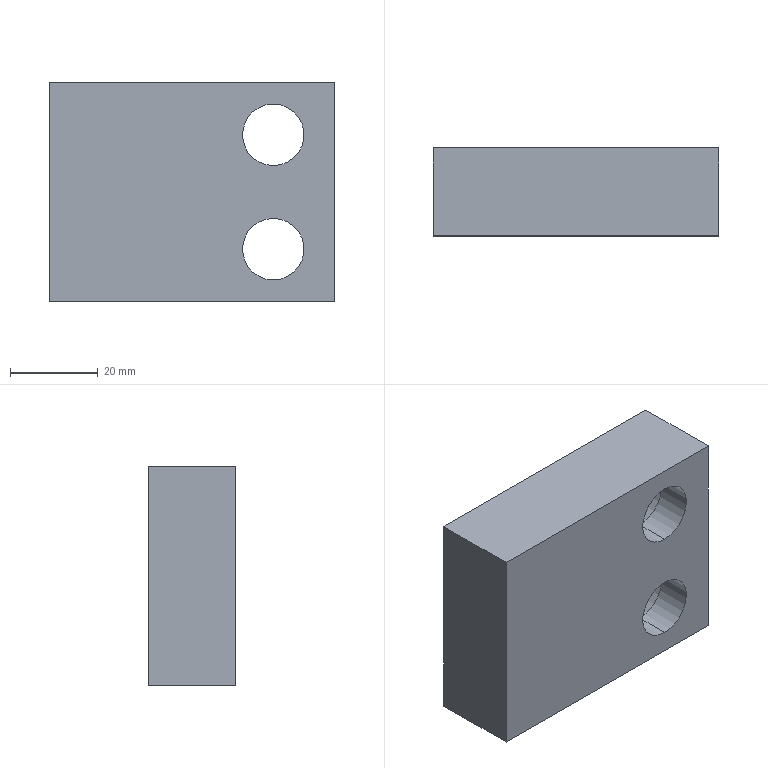Part | STEP file | OP10-026_stopper plate | 1 solid | 20 faces | box 65 x 20 x 50 mm | volume 54932 mm3 | cylinder 8 | plane 8 | cone 4 | commonest cylinder face diameters 14 x4 20 x4
STEP:
#1=CARTESIAN_POINT('',(0.,0.,0.));
#2=DIRECTION('',(0.,0.,1.));
#3=DIRECTION('',(1.,0.,0.));
#4=AXIS2_PLACEMENT_3D('',#1,#2,#3);
#5=CARTESIAN_POINT('',(18.5,19.,-3.));
#6=VERTEX_POINT('',#5);
#7=CARTESIAN_POINT('',(18.5,20.,-2.));
#8=VERTEX_POINT('',#7);
#9=CARTESIAN_POINT('',(18.5,19.,-3.));
#10=DIRECTION('',(0.,0.7071,0.7071));
#11=VECTOR('',#10,1.);
#12=LINE('',#9,#11);
#13=CARTESIAN_POINT('',(18.5,19.,-13.));
#14=DIRECTION('',(0.,1.,0.));
#15=DIRECTION('',(0.,0.,1.));
#16=AXIS2_PLACEMENT_3D('',#13,#14,#15);
#17=CONICAL_SURFACE('',#16,10.,0.7854);
#18=CARTESIAN_POINT('',(6.283,0.));
#19=DIRECTION('',(0.,1.));
#20=VECTOR('',#19,1.);
#21=LINE('',#18,#20);
#22=(GEOMETRIC_REPRESENTATION_CONTEXT(2)PARAMETRIC_REPRESENTATION_CONTEXT()REPRESENTATION_CONTEXT('',''));
#23=DEFINITIONAL_REPRESENTATION('',(#21),#22);
#24=PCURVE('',#17,#23);
#25=CARTESIAN_POINT('',(18.5,19.,-13.));
#26=DIRECTION('',(0.,1.,0.));
#27=DIRECTION('',(0.,0.,1.));
#28=AXIS2_PLACEMENT_3D('',#25,#26,#27);
#29=CONICAL_SURFACE('',#28,10.,0.7854);
#30=CARTESIAN_POINT('',(0.,0.));
#31=DIRECTION('',(0.,1.));
#32=VECTOR('',#31,1.);
#33=LINE('',#30,#32);
#34=(GEOMETRIC_REPRESENTATION_CONTEXT(2)PARAMETRIC_REPRESENTATION_CONTEXT()REPRESENTATION_CONTEXT('',''));
#35=DEFINITIONAL_REPRESENTATION('',(#33),#34);
#36=PCURVE('',#29,#35);
#37=SURFACE_CURVE('',#12,(#24,#36),.PCURVE_S1.);
#38=EDGE_CURVE('',#6,#8,#37,.T.);
#39=ORIENTED_EDGE('',*,*,#38,.T.);
#40=CARTESIAN_POINT('',(18.5,20.,-24.));
#41=VERTEX_POINT('',#40);
#42=CARTESIAN_POINT('',(18.5,20.,-13.));
#43=DIRECTION('',(0.,-1.,0.));
#44=DIRECTION('',(0.,0.,-1.));
#45=AXIS2_PLACEMENT_3D('',#42,#43,#44);
#46=CIRCLE('',#45,11.);
#47=CARTESIAN_POINT('',(9.425,1.));
#48=DIRECTION('',(-1.,0.));
#49=VECTOR('',#48,1.);
#50=LINE('',#47,#49);
#51=(GEOMETRIC_REPRESENTATION_CONTEXT(2)PARAMETRIC_REPRESENTATION_CONTEXT()REPRESENTATION_CONTEXT('',''));
#52=DEFINITIONAL_REPRESENTATION('',(#50),#51);
#53=PCURVE('',#17,#52);
#54=CARTESIAN_POINT('',(0.,20.,0.));
#55=DIRECTION('',(0.,-1.,0.));
#56=DIRECTION('',(0.,0.,-1.));
#57=AXIS2_PLACEMENT_3D('',#54,#55,#56);
#58=PLANE('',#57);
#59=CARTESIAN_POINT('',(13.,18.5));
#60=DIRECTION('',(1.,0.));
#61=AXIS2_PLACEMENT_2D('',#59,#60);
#62=CIRCLE('',#61,11.);
#63=(GEOMETRIC_REPRESENTATION_CONTEXT(2)PARAMETRIC_REPRESENTATION_CONTEXT()REPRESENTATION_CONTEXT('',''));
#64=DEFINITIONAL_REPRESENTATION('',(#62),#63);
#65=PCURVE('',#58,#64);
#66=SURFACE_CURVE('',#46,(#53,#65),.PCURVE_S1.);
#67=EDGE_CURVE('',#8,#41,#66,.T.);
#68=ORIENTED_EDGE('',*,*,#67,.T.);
#69=CARTESIAN_POINT('',(18.5,19.,-23.));
#70=VERTEX_POINT('',#69);
#71=CARTESIAN_POINT('',(18.5,19.,-23.));
#72=DIRECTION('',(0.,0.7071,-0.7071));
#73=VECTOR('',#72,1.);
#74=LINE('',#71,#73);
#75=CARTESIAN_POINT('',(3.142,0.));
#76=DIRECTION('',(0.,1.));
#77=VECTOR('',#76,1.);
#78=LINE('',#75,#77);
#79=(GEOMETRIC_REPRESENTATION_CONTEXT(2)PARAMETRIC_REPRESENTATION_CONTEXT()REPRESENTATION_CONTEXT('',''));
#80=DEFINITIONAL_REPRESENTATION('',(#78),#79);
#81=PCURVE('',#17,#80);
#82=CARTESIAN_POINT('',(3.142,0.));
#83=DIRECTION('',(0.,1.));
#84=VECTOR('',#83,1.);
#85=LINE('',#82,#84);
#86=(GEOMETRIC_REPRESENTATION_CONTEXT(2)PARAMETRIC_REPRESENTATION_CONTEXT()REPRESENTATION_CONTEXT('',''));
#87=DEFINITIONAL_REPRESENTATION('',(#85),#86);
#88=PCURVE('',#29,#87);
#89=SURFACE_CURVE('',#74,(#81,#88),.PCURVE_S1.);
#90=EDGE_CURVE('',#70,#41,#89,.T.);
#91=ORIENTED_EDGE('',*,*,#90,.F.);
#92=CARTESIAN_POINT('',(18.5,19.,-13.));
#93=DIRECTION('',(0.,1.,0.));
#94=DIRECTION('',(0.,0.,-1.));
#95=AXIS2_PLACEMENT_3D('',#92,#93,#94);
#96=CIRCLE('',#95,10.);
#97=CARTESIAN_POINT('',(3.142,0.));
#98=DIRECTION('',(1.,0.));
#99=VECTOR('',#98,1.);
#100=LINE('',#97,#99);
#101=(GEOMETRIC_REPRESENTATION_CONTEXT(2)PARAMETRIC_REPRESENTATION_CONTEXT()REPRESENTATION_CONTEXT('',''));
#102=DEFINITIONAL_REPRESENTATION('',(#100),#101);
#103=PCURVE('',#17,#102);
#104=CARTESIAN_POINT('',(18.5,20.,-13.));
#105=DIRECTION('',(0.,1.,0.));
#106=DIRECTION('',(0.,0.,1.));
#107=AXIS2_PLACEMENT_3D('',#104,#105,#106);
#108=CYLINDRICAL_SURFACE('',#107,10.);
#109=CARTESIAN_POINT('',(3.142,-1.));
#110=DIRECTION('',(1.,0.));
#111=VECTOR('',#110,1.);
#112=LINE('',#109,#111);
#113=(GEOMETRIC_REPRESENTATION_CONTEXT(2)PARAMETRIC_REPRESENTATION_CONTEXT()REPRESENTATION_CONTEXT('',''));
#114=DEFINITIONAL_REPRESENTATION('',(#112),#113);
#115=PCURVE('',#108,#114);
#116=SURFACE_CURVE('',#96,(#103,#115),.PCURVE_S1.);
#117=EDGE_CURVE('',#70,#6,#116,.T.);
#118=ORIENTED_EDGE('',*,*,#117,.T.);
#119=EDGE_LOOP('',(#39,#68,#91,#118));
#120=FACE_BOUND('',#119,.F.);
#121=ADVANCED_FACE('',(#120),#17,.F.);
#122=CARTESIAN_POINT('',(18.5,19.,23.));
#123=VERTEX_POINT('',#122);
#124=CARTESIAN_POINT('',(18.5,20.,24.));
#125=VERTEX_POINT('',#124);
#126=CARTESIAN_POINT('',(18.5,19.,23.));
#127=DIRECTION('',(0.,0.7071,0.7071));
#128=VECTOR('',#127,1.);
#129=LINE('',#126,#128);
#130=CARTESIAN_POINT('',(18.5,19.,13.));
#131=DIRECTION('',(0.,1.,0.));
#132=DIRECTION('',(0.,0.,1.));
#133=AXIS2_PLACEMENT_3D('',#130,#131,#132);
#134=CONICAL_SURFACE('',#133,10.,0.7854);
#135=CARTESIAN_POINT('',(6.283,0.));
#136=DIRECTION('',(0.,1.));
#137=VECTOR('',#136,1.);
#138=LINE('',#135,#137);
#139=(GEOMETRIC_REPRESENTATION_CONTEXT(2)PARAMETRIC_REPRESENTATION_CONTEXT()REPRESENTATION_CONTEXT('',''));
#140=DEFINITIONAL_REPRESENTATION('',(#138),#139);
#141=PCURVE('',#134,#140);
#142=CARTESIAN_POINT('',(18.5,19.,13.));
#143=DIRECTION('',(0.,1.,0.));
#144=DIRECTION('',(0.,0.,1.));
#145=AXIS2_PLACEMENT_3D('',#142,#143,#144);
#146=CONICAL_SURFACE('',#145,10.,0.7854);
#147=CARTESIAN_POINT('',(0.,0.));
#148=DIRECTION('',(0.,1.));
#149=VECTOR('',#148,1.);
#150=LINE('',#147,#149);
#151=(GEOMETRIC_REPRESENTATION_CONTEXT(2)PARAMETRIC_REPRESENTATION_CONTEXT()REPRESENTATION_CONTEXT('',''));
#152=DEFINITIONAL_REPRESENTATION('',(#150),#151);
#153=PCURVE('',#146,#152);
#154=SURFACE_CURVE('',#129,(#141,#153),.PCURVE_S1.);
#155=EDGE_CURVE('',#123,#125,#154,.T.);
#156=ORIENTED_EDGE('',*,*,#155,.T.);
#157=CARTESIAN_POINT('',(18.5,20.,2.));
#158=VERTEX_POINT('',#157);
#159=CARTESIAN_POINT('',(18.5,20.,13.));
#160=DIRECTION('',(0.,-1.,0.));
#161=DIRECTION('',(0.,0.,-1.));
#162=AXIS2_PLACEMENT_3D('',#159,#160,#161);
#163=CIRCLE('',#162,11.);
#164=CARTESIAN_POINT('',(9.425,1.));
#165=DIRECTION('',(-1.,0.));
#166=VECTOR('',#165,1.);
#167=LINE('',#164,#166);
#168=(GEOMETRIC_REPRESENTATION_CONTEXT(2)PARAMETRIC_REPRESENTATION_CONTEXT()REPRESENTATION_CONTEXT('',''));
#169=DEFINITIONAL_REPRESENTATION('',(#167),#168);
#170=PCURVE('',#134,#169);
#171=CARTESIAN_POINT('',(-13.,18.5));
#172=DIRECTION('',(1.,0.));
#173=AXIS2_PLACEMENT_2D('',#171,#172);
#174=CIRCLE('',#173,11.);
#175=(GEOMETRIC_REPRESENTATION_CONTEXT(2)PARAMETRIC_REPRESENTATION_CONTEXT()REPRESENTATION_CONTEXT('',''));
#176=DEFINITIONAL_REPRESENTATION('',(#174),#175);
#177=PCURVE('',#58,#176);
#178=SURFACE_CURVE('',#163,(#170,#177),.PCURVE_S1.);
#179=EDGE_CURVE('',#125,#158,#178,.T.);
#180=ORIENTED_EDGE('',*,*,#179,.T.);
#181=CARTESIAN_POINT('',(18.5,19.,3.));
#182=VERTEX_POINT('',#181);
#183=CARTESIAN_POINT('',(18.5,19.,3.));
#184=DIRECTION('',(0.,0.7071,-0.7071));
#185=VECTOR('',#184,1.);
#186=LINE('',#183,#185);
#187=CARTESIAN_POINT('',(3.142,0.));
#188=DIRECTION('',(0.,1.));
#189=VECTOR('',#188,1.);
#190=LINE('',#187,#189);
#191=(GEOMETRIC_REPRESENTATION_CONTEXT(2)PARAMETRIC_REPRESENTATION_CONTEXT()REPRESENTATION_CONTEXT('',''));
#192=DEFINITIONAL_REPRESENTATION('',(#190),#191);
#193=PCURVE('',#134,#192);
#194=CARTESIAN_POINT('',(3.142,0.));
#195=DIRECTION('',(0.,1.));
#196=VECTOR('',#195,1.);
#197=LINE('',#194,#196);
#198=(GEOMETRIC_REPRESENTATION_CONTEXT(2)PARAMETRIC_REPRESENTATION_CONTEXT()REPRESENTATION_CONTEXT('',''));
#199=DEFINITIONAL_REPRESENTATION('',(#197),#198);
#200=PCURVE('',#146,#199);
#201=SURFACE_CURVE('',#186,(#193,#200),.PCURVE_S1.);
#202=EDGE_CURVE('',#182,#158,#201,.T.);
#203=ORIENTED_EDGE('',*,*,#202,.F.);
#204=CARTESIAN_POINT('',(18.5,19.,13.));
#205=DIRECTION('',(0.,1.,0.));
#206=DIRECTION('',(0.,0.,-1.));
#207=AXIS2_PLACEMENT_3D('',#204,#205,#206);
#208=CIRCLE('',#207,10.);
#209=CARTESIAN_POINT('',(3.142,0.));
#210=DIRECTION('',(1.,0.));
#211=VECTOR('',#210,1.);
#212=LINE('',#209,#211);
#213=(GEOMETRIC_REPRESENTATION_CONTEXT(2)PARAMETRIC_REPRESENTATION_CONTEXT()REPRESENTATION_CONTEXT('',''));
#214=DEFINITIONAL_REPRESENTATION('',(#212),#213);
#215=PCURVE('',#134,#214);
#216=CARTESIAN_POINT('',(18.5,20.,13.));
#217=DIRECTION('',(0.,1.,0.));
#218=DIRECTION('',(0.,0.,1.));
#219=AXIS2_PLACEMENT_3D('',#216,#217,#218);
#220=CYLINDRICAL_SURFACE('',#219,10.);
#221=CARTESIAN_POINT('',(3.142,-1.));
#222=DIRECTION('',(1.,0.));
#223=VECTOR('',#222,1.);
#224=LINE('',#221,#223);
#225=(GEOMETRIC_REPRESENTATION_CONTEXT(2)PARAMETRIC_REPRESENTATION_CONTEXT()REPRESENTATION_CONTEXT('',''));
#226=DEFINITIONAL_REPRESENTATION('',(#224),#225);
#227=PCURVE('',#220,#226);
#228=SURFACE_CURVE('',#208,(#215,#227),.PCURVE_S1.);
#229=EDGE_CURVE('',#182,#123,#228,.T.);
#230=ORIENTED_EDGE('',*,*,#229,.T.);
#231=EDGE_LOOP('',(#156,#180,#203,#230));
#232=FACE_BOUND('',#231,.F.);
#233=ADVANCED_FACE('',(#232),#134,.F.);
#234=CARTESIAN_POINT('',(18.5,8.,23.));
#235=VERTEX_POINT('',#234);
#236=CARTESIAN_POINT('',(18.5,20.,23.));
#237=DIRECTION('',(0.,1.,0.));
#238=VECTOR('',#237,1.);
#239=LINE('',#236,#238);
#240=CARTESIAN_POINT('',(6.283,0.));
#241=DIRECTION('',(0.,1.));
#242=VECTOR('',#241,1.);
#243=LINE('',#240,#242);
#244=(GEOMETRIC_REPRESENTATION_CONTEXT(2)PARAMETRIC_REPRESENTATION_CONTEXT()REPRESENTATION_CONTEXT('',''));
#245=DEFINITIONAL_REPRESENTATION('',(#243),#244);
#246=PCURVE('',#220,#245);
#247=CARTESIAN_POINT('',(18.5,20.,13.));
#248=DIRECTION('',(0.,1.,0.));
#249=DIRECTION('',(0.,0.,1.));
#250=AXIS2_PLACEMENT_3D('',#247,#248,#249);
#251=CYLINDRICAL_SURFACE('',#250,10.);
#252=CARTESIAN_POINT('',(0.,0.));
#253=DIRECTION('',(0.,1.));
#254=VECTOR('',#253,1.);
#255=LINE('',#252,#254);
#256=(GEOMETRIC_REPRESENTATION_CONTEXT(2)PARAMETRIC_REPRESENTATION_CONTEXT()REPRESENTATION_CONTEXT('',''));
#257=DEFINITIONAL_REPRESENTATION('',(#255),#256);
#258=PCURVE('',#251,#257);
#259=SURFACE_CURVE('',#239,(#246,#258),.PCURVE_S1.);
#260=EDGE_CURVE('',#235,#123,#259,.T.);
#261=ORIENTED_EDGE('',*,*,#260,.T.);
#262=ORIENTED_EDGE('',*,*,#229,.F.);
#263=CARTESIAN_POINT('',(18.5,8.,3.));
#264=VERTEX_POINT('',#263);
#265=CARTESIAN_POINT('',(18.5,20.,3.));
#266=DIRECTION('',(0.,1.,0.));
#267=VECTOR('',#266,1.);
#268=LINE('',#265,#267);
#269=CARTESIAN_POINT('',(3.142,0.));
#270=DIRECTION('',(0.,1.));
#271=VECTOR('',#270,1.);
#272=LINE('',#269,#271);
#273=(GEOMETRIC_REPRESENTATION_CONTEXT(2)PARAMETRIC_REPRESENTATION_CONTEXT()REPRESENTATION_CONTEXT('',''));
#274=DEFINITIONAL_REPRESENTATION('',(#272),#273);
#275=PCURVE('',#220,#274);
#276=CARTESIAN_POINT('',(3.142,0.));
#277=DIRECTION('',(0.,1.));
#278=VECTOR('',#277,1.);
#279=LINE('',#276,#278);
#280=(GEOMETRIC_REPRESENTATION_CONTEXT(2)PARAMETRIC_REPRESENTATION_CONTEXT()REPRESENTATION_CONTEXT('',''));
#281=DEFINITIONAL_REPRESENTATION('',(#279),#280);
#282=PCURVE('',#251,#281);
#283=SURFACE_CURVE('',#268,(#275,#282),.PCURVE_S1.);
#284=EDGE_CURVE('',#264,#182,#283,.T.);
#285=ORIENTED_EDGE('',*,*,#284,.F.);
#286=CARTESIAN_POINT('',(18.5,8.,13.));
#287=DIRECTION('',(0.,1.,0.));
#288=DIRECTION('',(0.,0.,1.));
#289=AXIS2_PLACEMENT_3D('',#286,#287,#288);
#290=CIRCLE('',#289,10.);
#291=CARTESIAN_POINT('',(0.,-12.));
#292=DIRECTION('',(1.,0.));
#293=VECTOR('',#292,1.);
#294=LINE('',#291,#293);
#295=(GEOMETRIC_REPRESENTATION_CONTEXT(2)PARAMETRIC_REPRESENTATION_CONTEXT()REPRESENTATION_CONTEXT('',''));
#296=DEFINITIONAL_REPRESENTATION('',(#294),#295);
#297=PCURVE('',#220,#296);
#298=CARTESIAN_POINT('',(25.5,8.,13.));
#299=DIRECTION('',(0.,-1.,0.));
#300=DIRECTION('',(0.,0.,-1.));
#301=AXIS2_PLACEMENT_3D('',#298,#299,#300);
#302=PLANE('',#301);
#303=CARTESIAN_POINT('',(-10.,-7.));
#304=CARTESIAN_POINT('',(-10.,10.321));
#305=CARTESIAN_POINT('',(5.,1.66));
#306=CARTESIAN_POINT('',(20.,-7.));
#307=CARTESIAN_POINT('',(5.,-15.66));
#308=CARTESIAN_POINT('',(-10.,-24.321));
#309=CARTESIAN_POINT('',(-10.,-7.));
#310=(BOUNDED_CURVE()B_SPLINE_CURVE(2,(#303,#304,#305,#306,#307,#308,#309),.UNSPECIFIED.,.T.,.F.)B_SPLINE_CURVE_WITH_KNOTS((1,2,2,2,2,1),(-2.094,0.,2.094,4.189,6.283,8.378),.UNSPECIFIED.)CURVE()GEOMETRIC_REPRESENTATION_ITEM()RATIONAL_B_SPLINE_CURVE((1.,0.5,1.,0.5,1.,0.5,1.))REPRESENTATION_ITEM(''));
#311=(GEOMETRIC_REPRESENTATION_CONTEXT(2)PARAMETRIC_REPRESENTATION_CONTEXT()REPRESENTATION_CONTEXT('',''));
#312=DEFINITIONAL_REPRESENTATION('',(#310),#311);
#313=PCURVE('',#302,#312);
#314=SURFACE_CURVE('',#290,(#297,#313),.PCURVE_S1.);
#315=EDGE_CURVE('',#264,#235,#314,.T.);
#316=ORIENTED_EDGE('',*,*,#315,.T.);
#317=EDGE_LOOP('',(#261,#262,#285,#316));
#318=FACE_BOUND('',#317,.F.);
#319=ADVANCED_FACE('',(#318),#220,.F.);
#320=CARTESIAN_POINT('',(18.5,0.,20.));
#321=VERTEX_POINT('',#320);
#322=CARTESIAN_POINT('',(18.5,8.,20.));
#323=VERTEX_POINT('',#322);
#324=CARTESIAN_POINT('',(18.5,20.,20.));
#325=DIRECTION('',(0.,1.,0.));
#326=VECTOR('',#325,1.);
#327=LINE('',#324,#326);
#328=CARTESIAN_POINT('',(18.5,20.,13.));
#329=DIRECTION('',(0.,1.,0.));
#330=DIRECTION('',(0.,0.,1.));
#331=AXIS2_PLACEMENT_3D('',#328,#329,#330);
#332=CYLINDRICAL_SURFACE('',#331,7.);
#333=CARTESIAN_POINT('',(6.283,0.));
#334=DIRECTION('',(0.,1.));
#335=VECTOR('',#334,1.);
#336=LINE('',#333,#335);
#337=(GEOMETRIC_REPRESENTATION_CONTEXT(2)PARAMETRIC_REPRESENTATION_CONTEXT()REPRESENTATION_CONTEXT('',''));
#338=DEFINITIONAL_REPRESENTATION('',(#336),#337);
#339=PCURVE('',#332,#338);
#340=CARTESIAN_POINT('',(18.5,20.,13.));
#341=DIRECTION('',(0.,1.,0.));
#342=DIRECTION('',(0.,0.,1.));
#343=AXIS2_PLACEMENT_3D('',#340,#341,#342);
#344=CYLINDRICAL_SURFACE('',#343,7.);
#345=CARTESIAN_POINT('',(0.,0.));
#346=DIRECTION('',(0.,1.));
#347=VECTOR('',#346,1.);
#348=LINE('',#345,#347);
#349=(GEOMETRIC_REPRESENTATION_CONTEXT(2)PARAMETRIC_REPRESENTATION_CONTEXT()REPRESENTATION_CONTEXT('',''));
#350=DEFINITIONAL_REPRESENTATION('',(#348),#349);
#351=PCURVE('',#344,#350);
#352=SURFACE_CURVE('',#327,(#339,#351),.PCURVE_S1.);
#353=EDGE_CURVE('',#321,#323,#352,.T.);
#354=ORIENTED_EDGE('',*,*,#353,.T.);
#355=CARTESIAN_POINT('',(18.5,8.,6.));
#356=VERTEX_POINT('',#355);
#357=CARTESIAN_POINT('',(18.5,8.,13.));
#358=DIRECTION('',(0.,1.,0.));
#359=DIRECTION('',(0.,0.,1.));
#360=AXIS2_PLACEMENT_3D('',#357,#358,#359);
#361=CIRCLE('',#360,7.);
#362=CARTESIAN_POINT('',(0.,-12.));
#363=DIRECTION('',(1.,0.));
#364=VECTOR('',#363,1.);
#365=LINE('',#362,#364);
#366=(GEOMETRIC_REPRESENTATION_CONTEXT(2)PARAMETRIC_REPRESENTATION_CONTEXT()REPRESENTATION_CONTEXT('',''));
#367=DEFINITIONAL_REPRESENTATION('',(#365),#366);
#368=PCURVE('',#332,#367);
#369=CARTESIAN_POINT('',(-7.,-7.));
#370=CARTESIAN_POINT('',(-7.,5.124));
#371=CARTESIAN_POINT('',(3.5,-0.9378));
#372=CARTESIAN_POINT('',(14.,-7.));
#373=CARTESIAN_POINT('',(3.5,-13.062));
#374=CARTESIAN_POINT('',(-7.,-19.124));
#375=CARTESIAN_POINT('',(-7.,-7.));
#376=(BOUNDED_CURVE()B_SPLINE_CURVE(2,(#369,#370,#371,#372,#373,#374,#375),.UNSPECIFIED.,.T.,.F.)B_SPLINE_CURVE_WITH_KNOTS((1,2,2,2,2,1),(-2.094,0.,2.094,4.189,6.283,8.378),.UNSPECIFIED.)CURVE()GEOMETRIC_REPRESENTATION_ITEM()RATIONAL_B_SPLINE_CURVE((1.,0.5,1.,0.5,1.,0.5,1.))REPRESENTATION_ITEM(''));
#377=(GEOMETRIC_REPRESENTATION_CONTEXT(2)PARAMETRIC_REPRESENTATION_CONTEXT()REPRESENTATION_CONTEXT('',''));
#378=DEFINITIONAL_REPRESENTATION('',(#376),#377);
#379=PCURVE('',#302,#378);
#380=SURFACE_CURVE('',#361,(#368,#379),.PCURVE_S1.);
#381=EDGE_CURVE('',#356,#323,#380,.T.);
#382=ORIENTED_EDGE('',*,*,#381,.F.);
#383=CARTESIAN_POINT('',(18.5,0.,6.));
#384=VERTEX_POINT('',#383);
#385=CARTESIAN_POINT('',(18.5,20.,6.));
#386=DIRECTION('',(0.,1.,0.));
#387=VECTOR('',#386,1.);
#388=LINE('',#385,#387);
#389=CARTESIAN_POINT('',(3.142,0.));
#390=DIRECTION('',(0.,1.));
#391=VECTOR('',#390,1.);
#392=LINE('',#389,#391);
#393=(GEOMETRIC_REPRESENTATION_CONTEXT(2)PARAMETRIC_REPRESENTATION_CONTEXT()REPRESENTATION_CONTEXT('',''));
#394=DEFINITIONAL_REPRESENTATION('',(#392),#393);
#395=PCURVE('',#332,#394);
#396=CARTESIAN_POINT('',(3.142,0.));
#397=DIRECTION('',(0.,1.));
#398=VECTOR('',#397,1.);
#399=LINE('',#396,#398);
#400=(GEOMETRIC_REPRESENTATION_CONTEXT(2)PARAMETRIC_REPRESENTATION_CONTEXT()REPRESENTATION_CONTEXT('',''));
#401=DEFINITIONAL_REPRESENTATION('',(#399),#400);
#402=PCURVE('',#344,#401);
#403=SURFACE_CURVE('',#388,(#395,#402),.PCURVE_S1.);
#404=EDGE_CURVE('',#384,#356,#403,.T.);
#405=ORIENTED_EDGE('',*,*,#404,.F.);
#406=CARTESIAN_POINT('',(18.5,0.,13.));
#407=DIRECTION('',(0.,1.,0.));
#408=DIRECTION('',(0.,0.,1.));
#409=AXIS2_PLACEMENT_3D('',#406,#407,#408);
#410=CIRCLE('',#409,7.);
#411=CARTESIAN_POINT('',(0.,-20.));
#412=DIRECTION('',(1.,0.));
#413=VECTOR('',#412,1.);
#414=LINE('',#411,#413);
#415=(GEOMETRIC_REPRESENTATION_CONTEXT(2)PARAMETRIC_REPRESENTATION_CONTEXT()REPRESENTATION_CONTEXT('',''));
#416=DEFINITIONAL_REPRESENTATION('',(#414),#415);
#417=PCURVE('',#332,#416);
#418=CARTESIAN_POINT('',(0.,0.,0.));
#419=DIRECTION('',(0.,-1.,0.));
#420=DIRECTION('',(0.,0.,-1.));
#421=AXIS2_PLACEMENT_3D('',#418,#419,#420);
#422=PLANE('',#421);
#423=CARTESIAN_POINT('',(-20.,18.5));
#424=CARTESIAN_POINT('',(-20.,30.624));
#425=CARTESIAN_POINT('',(-9.5,24.562));
#426=CARTESIAN_POINT('',(1.,18.5));
#427=CARTESIAN_POINT('',(-9.5,12.438));
#428=CARTESIAN_POINT('',(-20.,6.376));
#429=CARTESIAN_POINT('',(-20.,18.5));
#430=(BOUNDED_CURVE()B_SPLINE_CURVE(2,(#423,#424,#425,#426,#427,#428,#429),.UNSPECIFIED.,.T.,.F.)B_SPLINE_CURVE_WITH_KNOTS((1,2,2,2,2,1),(-2.094,0.,2.094,4.189,6.283,8.378),.UNSPECIFIED.)CURVE()GEOMETRIC_REPRESENTATION_ITEM()RATIONAL_B_SPLINE_CURVE((1.,0.5,1.,0.5,1.,0.5,1.))REPRESENTATION_ITEM(''));
#431=(GEOMETRIC_REPRESENTATION_CONTEXT(2)PARAMETRIC_REPRESENTATION_CONTEXT()REPRESENTATION_CONTEXT('',''));
#432=DEFINITIONAL_REPRESENTATION('',(#430),#431);
#433=PCURVE('',#422,#432);
#434=SURFACE_CURVE('',#410,(#417,#433),.PCURVE_S1.);
#435=EDGE_CURVE('',#384,#321,#434,.T.);
#436=ORIENTED_EDGE('',*,*,#435,.T.);
#437=EDGE_LOOP('',(#354,#382,#405,#436));
#438=FACE_BOUND('',#437,.F.);
#439=ADVANCED_FACE('',(#438),#332,.F.);
#440=CARTESIAN_POINT('',(18.5,8.,-3.));
#441=VERTEX_POINT('',#440);
#442=CARTESIAN_POINT('',(18.5,20.,-3.));
#443=DIRECTION('',(0.,1.,0.));
#444=VECTOR('',#443,1.);
#445=LINE('',#442,#444);
#446=CARTESIAN_POINT('',(6.283,0.));
#447=DIRECTION('',(0.,1.));
#448=VECTOR('',#447,1.);
#449=LINE('',#446,#448);
#450=(GEOMETRIC_REPRESENTATION_CONTEXT(2)PARAMETRIC_REPRESENTATION_CONTEXT()REPRESENTATION_CONTEXT('',''));
#451=DEFINITIONAL_REPRESENTATION('',(#449),#450);
#452=PCURVE('',#108,#451);
#453=CARTESIAN_POINT('',(18.5,20.,-13.));
#454=DIRECTION('',(0.,1.,0.));
#455=DIRECTION('',(0.,0.,1.));
#456=AXIS2_PLACEMENT_3D('',#453,#454,#455);
#457=CYLINDRICAL_SURFACE('',#456,10.);
#458=CARTESIAN_POINT('',(0.,0.));
#459=DIRECTION('',(0.,1.));
#460=VECTOR('',#459,1.);
#461=LINE('',#458,#460);
#462=(GEOMETRIC_REPRESENTATION_CONTEXT(2)PARAMETRIC_REPRESENTATION_CONTEXT()REPRESENTATION_CONTEXT('',''));
#463=DEFINITIONAL_REPRESENTATION('',(#461),#462);
#464=PCURVE('',#457,#463);
#465=SURFACE_CURVE('',#445,(#452,#464),.PCURVE_S1.);
#466=EDGE_CURVE('',#441,#6,#465,.T.);
#467=ORIENTED_EDGE('',*,*,#466,.T.);
#468=ORIENTED_EDGE('',*,*,#117,.F.);
#469=CARTESIAN_POINT('',(18.5,8.,-23.));
#470=VERTEX_POINT('',#469);
#471=CARTESIAN_POINT('',(18.5,20.,-23.));
#472=DIRECTION('',(0.,1.,0.));
#473=VECTOR('',#472,1.);
#474=LINE('',#471,#473);
#475=CARTESIAN_POINT('',(3.142,0.));
#476=DIRECTION('',(0.,1.));
#477=VECTOR('',#476,1.);
#478=LINE('',#475,#477);
#479=(GEOMETRIC_REPRESENTATION_CONTEXT(2)PARAMETRIC_REPRESENTATION_CONTEXT()REPRESENTATION_CONTEXT('',''));
#480=DEFINITIONAL_REPRESENTATION('',(#478),#479);
#481=PCURVE('',#108,#480);
#482=CARTESIAN_POINT('',(3.142,0.));
#483=DIRECTION('',(0.,1.));
#484=VECTOR('',#483,1.);
#485=LINE('',#482,#484);
#486=(GEOMETRIC_REPRESENTATION_CONTEXT(2)PARAMETRIC_REPRESENTATION_CONTEXT()REPRESENTATION_CONTEXT('',''));
#487=DEFINITIONAL_REPRESENTATION('',(#485),#486);
#488=PCURVE('',#457,#487);
#489=SURFACE_CURVE('',#474,(#481,#488),.PCURVE_S1.);
#490=EDGE_CURVE('',#470,#70,#489,.T.);
#491=ORIENTED_EDGE('',*,*,#490,.F.);
#492=CARTESIAN_POINT('',(18.5,8.,-13.));
#493=DIRECTION('',(0.,1.,0.));
#494=DIRECTION('',(0.,0.,1.));
#495=AXIS2_PLACEMENT_3D('',#492,#493,#494);
#496=CIRCLE('',#495,10.);
#497=CARTESIAN_POINT('',(0.,-12.));
#498=DIRECTION('',(1.,0.));
#499=VECTOR('',#498,1.);
#500=LINE('',#497,#499);
#501=(GEOMETRIC_REPRESENTATION_CONTEXT(2)PARAMETRIC_REPRESENTATION_CONTEXT()REPRESENTATION_CONTEXT('',''));
#502=DEFINITIONAL_REPRESENTATION('',(#500),#501);
#503=PCURVE('',#108,#502);
#504=CARTESIAN_POINT('',(25.5,8.,-13.));
#505=DIRECTION('',(0.,-1.,0.));
#506=DIRECTION('',(0.,0.,-1.));
#507=AXIS2_PLACEMENT_3D('',#504,#505,#506);
#508=PLANE('',#507);
#509=CARTESIAN_POINT('',(-10.,-7.));
#510=CARTESIAN_POINT('',(-10.,10.321));
#511=CARTESIAN_POINT('',(5.,1.66));
#512=CARTESIAN_POINT('',(20.,-7.));
#513=CARTESIAN_POINT('',(5.,-15.66));
#514=CARTESIAN_POINT('',(-10.,-24.321));
#515=CARTESIAN_POINT('',(-10.,-7.));
#516=(BOUNDED_CURVE()B_SPLINE_CURVE(2,(#509,#510,#511,#512,#513,#514,#515),.UNSPECIFIED.,.T.,.F.)B_SPLINE_CURVE_WITH_KNOTS((1,2,2,2,2,1),(-2.094,0.,2.094,4.189,6.283,8.378),.UNSPECIFIED.)CURVE()GEOMETRIC_REPRESENTATION_ITEM()RATIONAL_B_SPLINE_CURVE((1.,0.5,1.,0.5,1.,0.5,1.))REPRESENTATION_ITEM(''));
#517=(GEOMETRIC_REPRESENTATION_CONTEXT(2)PARAMETRIC_REPRESENTATION_CONTEXT()REPRESENTATION_CONTEXT('',''));
#518=DEFINITIONAL_REPRESENTATION('',(#516),#517);
#519=PCURVE('',#508,#518);
#520=SURFACE_CURVE('',#496,(#503,#519),.PCURVE_S1.);
#521=EDGE_CURVE('',#470,#441,#520,.T.);
#522=ORIENTED_EDGE('',*,*,#521,.T.);
#523=EDGE_LOOP('',(#467,#468,#491,#522));
#524=FACE_BOUND('',#523,.F.);
#525=ADVANCED_FACE('',(#524),#108,.F.);
#526=CARTESIAN_POINT('',(18.5,0.,-6.));
#527=VERTEX_POINT('',#526);
#528=CARTESIAN_POINT('',(18.5,8.,-6.));
#529=VERTEX_POINT('',#528);
#530=CARTESIAN_POINT('',(18.5,20.,-6.));
#531=DIRECTION('',(0.,1.,0.));
#532=VECTOR('',#531,1.);
#533=LINE('',#530,#532);
#534=CARTESIAN_POINT('',(18.5,20.,-13.));
#535=DIRECTION('',(0.,1.,0.));
#536=DIRECTION('',(0.,0.,1.));
#537=AXIS2_PLACEMENT_3D('',#534,#535,#536);
#538=CYLINDRICAL_SURFACE('',#537,7.);
#539=CARTESIAN_POINT('',(6.283,0.));
#540=DIRECTION('',(0.,1.));
#541=VECTOR('',#540,1.);
#542=LINE('',#539,#541);
#543=(GEOMETRIC_REPRESENTATION_CONTEXT(2)PARAMETRIC_REPRESENTATION_CONTEXT()REPRESENTATION_CONTEXT('',''));
#544=DEFINITIONAL_REPRESENTATION('',(#542),#543);
#545=PCURVE('',#538,#544);
#546=CARTESIAN_POINT('',(18.5,20.,-13.));
#547=DIRECTION('',(0.,1.,0.));
#548=DIRECTION('',(0.,0.,1.));
#549=AXIS2_PLACEMENT_3D('',#546,#547,#548);
#550=CYLINDRICAL_SURFACE('',#549,7.);
#551=CARTESIAN_POINT('',(0.,0.));
#552=DIRECTION('',(0.,1.));
#553=VECTOR('',#552,1.);
#554=LINE('',#551,#553);
#555=(GEOMETRIC_REPRESENTATION_CONTEXT(2)PARAMETRIC_REPRESENTATION_CONTEXT()REPRESENTATION_CONTEXT('',''));
#556=DEFINITIONAL_REPRESENTATION('',(#554),#555);
#557=PCURVE('',#550,#556);
#558=SURFACE_CURVE('',#533,(#545,#557),.PCURVE_S1.);
#559=EDGE_CURVE('',#527,#529,#558,.T.);
#560=ORIENTED_EDGE('',*,*,#559,.T.);
#561=CARTESIAN_POINT('',(18.5,8.,-20.));
#562=VERTEX_POINT('',#561);
#563=CARTESIAN_POINT('',(18.5,8.,-13.));
#564=DIRECTION('',(0.,1.,0.));
#565=DIRECTION('',(0.,0.,1.));
#566=AXIS2_PLACEMENT_3D('',#563,#564,#565);
#567=CIRCLE('',#566,7.);
#568=CARTESIAN_POINT('',(0.,-12.));
#569=DIRECTION('',(1.,0.));
#570=VECTOR('',#569,1.);
#571=LINE('',#568,#570);
#572=(GEOMETRIC_REPRESENTATION_CONTEXT(2)PARAMETRIC_REPRESENTATION_CONTEXT()REPRESENTATION_CONTEXT('',''));
#573=DEFINITIONAL_REPRESENTATION('',(#571),#572);
#574=PCURVE('',#538,#573);
#575=CARTESIAN_POINT('',(-7.,-7.));
#576=CARTESIAN_POINT('',(-7.,5.124));
#577=CARTESIAN_POINT('',(3.5,-0.9378));
#578=CARTESIAN_POINT('',(14.,-7.));
#579=CARTESIAN_POINT('',(3.5,-13.062));
#580=CARTESIAN_POINT('',(-7.,-19.124));
#581=CARTESIAN_POINT('',(-7.,-7.));
#582=(BOUNDED_CURVE()B_SPLINE_CURVE(2,(#575,#576,#577,#578,#579,#580,#581),.UNSPECIFIED.,.T.,.F.)B_SPLINE_CURVE_WITH_KNOTS((1,2,2,2,2,1),(-2.094,0.,2.094,4.189,6.283,8.378),.UNSPECIFIED.)CURVE()GEOMETRIC_REPRESENTATION_ITEM()RATIONAL_B_SPLINE_CURVE((1.,0.5,1.,0.5,1.,0.5,1.))REPRESENTATION_ITEM(''));
#583=(GEOMETRIC_REPRESENTATION_CONTEXT(2)PARAMETRIC_REPRESENTATION_CONTEXT()REPRESENTATION_CONTEXT('',''));
#584=DEFINITIONAL_REPRESENTATION('',(#582),#583);
#585=PCURVE('',#508,#584);
#586=SURFACE_CURVE('',#567,(#574,#585),.PCURVE_S1.);
#587=EDGE_CURVE('',#562,#529,#586,.T.);
#588=ORIENTED_EDGE('',*,*,#587,.F.);
#589=CARTESIAN_POINT('',(18.5,0.,-20.));
#590=VERTEX_POINT('',#589);
#591=CARTESIAN_POINT('',(18.5,20.,-20.));
#592=DIRECTION('',(0.,1.,0.));
#593=VECTOR('',#592,1.);
#594=LINE('',#591,#593);
#595=CARTESIAN_POINT('',(3.142,0.));
#596=DIRECTION('',(0.,1.));
#597=VECTOR('',#596,1.);
#598=LINE('',#595,#597);
#599=(GEOMETRIC_REPRESENTATION_CONTEXT(2)PARAMETRIC_REPRESENTATION_CONTEXT()REPRESENTATION_CONTEXT('',''));
#600=DEFINITIONAL_REPRESENTATION('',(#598),#599);
#601=PCURVE('',#538,#600);
#602=CARTESIAN_POINT('',(3.142,0.));
#603=DIRECTION('',(0.,1.));
#604=VECTOR('',#603,1.);
#605=LINE('',#602,#604);
#606=(GEOMETRIC_REPRESENTATION_CONTEXT(2)PARAMETRIC_REPRESENTATION_CONTEXT()REPRESENTATION_CONTEXT('',''));
#607=DEFINITIONAL_REPRESENTATION('',(#605),#606);
#608=PCURVE('',#550,#607);
#609=SURFACE_CURVE('',#594,(#601,#608),.PCURVE_S1.);
#610=EDGE_CURVE('',#590,#562,#609,.T.);
#611=ORIENTED_EDGE('',*,*,#610,.F.);
#612=CARTESIAN_POINT('',(18.5,0.,-13.));
#613=DIRECTION('',(0.,1.,0.));
#614=DIRECTION('',(0.,0.,1.));
#615=AXIS2_PLACEMENT_3D('',#612,#613,#614);
#616=CIRCLE('',#615,7.);
#617=CARTESIAN_POINT('',(0.,-20.));
#618=DIRECTION('',(1.,0.));
#619=VECTOR('',#618,1.);
#620=LINE('',#617,#619);
#621=(GEOMETRIC_REPRESENTATION_CONTEXT(2)PARAMETRIC_REPRESENTATION_CONTEXT()REPRESENTATION_CONTEXT('',''));
#622=DEFINITIONAL_REPRESENTATION('',(#620),#621);
#623=PCURVE('',#538,#622);
#624=CARTESIAN_POINT('',(6.,18.5));
#625=CARTESIAN_POINT('',(6.,30.624));
#626=CARTESIAN_POINT('',(16.5,24.562));
#627=CARTESIAN_POINT('',(27.,18.5));
#628=CARTESIAN_POINT('',(16.5,12.438));
#629=CARTESIAN_POINT('',(6.,6.376));
#630=CARTESIAN_POINT('',(6.,18.5));
#631=(BOUNDED_CURVE()B_SPLINE_CURVE(2,(#624,#625,#626,#627,#628,#629,#630),.UNSPECIFIED.,.T.,.F.)B_SPLINE_CURVE_WITH_KNOTS((1,2,2,2,2,1),(-2.094,0.,2.094,4.189,6.283,8.378),.UNSPECIFIED.)CURVE()GEOMETRIC_REPRESENTATION_ITEM()RATIONAL_B_SPLINE_CURVE((1.,0.5,1.,0.5,1.,0.5,1.))REPRESENTATION_ITEM(''));
#632=(GEOMETRIC_REPRESENTATION_CONTEXT(2)PARAMETRIC_REPRESENTATION_CONTEXT()REPRESENTATION_CONTEXT('',''));
#633=DEFINITIONAL_REPRESENTATION('',(#631),#632);
#634=PCURVE('',#422,#633);
#635=SURFACE_CURVE('',#616,(#623,#634),.PCURVE_S1.);
#636=EDGE_CURVE('',#590,#527,#635,.T.);
#637=ORIENTED_EDGE('',*,*,#636,.T.);
#638=EDGE_LOOP('',(#560,#588,#611,#637));
#639=FACE_BOUND('',#638,.F.);
#640=ADVANCED_FACE('',(#639),#538,.F.);
#641=CARTESIAN_POINT('',(32.5,0.,25.));
#642=VERTEX_POINT('',#641);
#643=CARTESIAN_POINT('',(32.5,0.,-25.));
#644=VERTEX_POINT('',#643);
#645=CARTESIAN_POINT('',(32.5,0.,25.));
#646=DIRECTION('',(0.,0.,-1.));
#647=VECTOR('',#646,1.);
#648=LINE('',#645,#647);
#649=CARTESIAN_POINT('',(32.5,20.,25.));
#650=DIRECTION('',(-1.,0.,0.));
#651=DIRECTION('',(0.,0.,1.));
#652=AXIS2_PLACEMENT_3D('',#649,#650,#651);
#653=PLANE('',#652);
#654=CARTESIAN_POINT('',(0.,-20.));
#655=DIRECTION('',(-1.,0.));
#656=VECTOR('',#655,1.);
#657=LINE('',#654,#656);
#658=(GEOMETRIC_REPRESENTATION_CONTEXT(2)PARAMETRIC_REPRESENTATION_CONTEXT()REPRESENTATION_CONTEXT('',''));
#659=DEFINITIONAL_REPRESENTATION('',(#657),#658);
#660=PCURVE('',#653,#659);
#661=CARTESIAN_POINT('',(-25.,32.5));
#662=DIRECTION('',(1.,0.));
#663=VECTOR('',#662,1.);
#664=LINE('',#661,#663);
#665=(GEOMETRIC_REPRESENTATION_CONTEXT(2)PARAMETRIC_REPRESENTATION_CONTEXT()REPRESENTATION_CONTEXT('',''));
#666=DEFINITIONAL_REPRESENTATION('',(#664),#665);
#667=PCURVE('',#422,#666);
#668=SURFACE_CURVE('',#648,(#660,#667),.PCURVE_S1.);
#669=EDGE_CURVE('',#642,#644,#668,.T.);
#670=ORIENTED_EDGE('',*,*,#669,.T.);
#671=CARTESIAN_POINT('',(32.5,20.,-25.));
#672=VERTEX_POINT('',#671);
#673=CARTESIAN_POINT('',(32.5,20.,-25.));
#674=DIRECTION('',(0.,-1.,0.));
#675=VECTOR('',#674,1.);
#676=LINE('',#673,#675);
#677=CARTESIAN_POINT('',(-50.,0.));
#678=DIRECTION('',(0.,-1.));
#679=VECTOR('',#678,1.);
#680=LINE('',#677,#679);
#681=(GEOMETRIC_REPRESENTATION_CONTEXT(2)PARAMETRIC_REPRESENTATION_CONTEXT()REPRESENTATION_CONTEXT('',''));
#682=DEFINITIONAL_REPRESENTATION('',(#680),#681);
#683=PCURVE('',#653,#682);
#684=CARTESIAN_POINT('',(-32.5,20.,-25.));
#685=DIRECTION('',(0.,0.,1.));
#686=DIRECTION('',(1.,0.,0.));
#687=AXIS2_PLACEMENT_3D('',#684,#685,#686);
#688=PLANE('',#687);
#689=CARTESIAN_POINT('',(65.,0.));
#690=DIRECTION('',(0.,-1.));
#691=VECTOR('',#690,1.);
#692=LINE('',#689,#691);
#693=(GEOMETRIC_REPRESENTATION_CONTEXT(2)PARAMETRIC_REPRESENTATION_CONTEXT()REPRESENTATION_CONTEXT('',''));
#694=DEFINITIONAL_REPRESENTATION('',(#692),#693);
#695=PCURVE('',#688,#694);
#696=SURFACE_CURVE('',#676,(#683,#695),.PCURVE_S1.);
#697=EDGE_CURVE('',#672,#644,#696,.T.);
#698=ORIENTED_EDGE('',*,*,#697,.F.);
#699=CARTESIAN_POINT('',(32.5,20.,25.));
#700=VERTEX_POINT('',#699);
#701=CARTESIAN_POINT('',(32.5,20.,25.));
#702=DIRECTION('',(0.,0.,-1.));
#703=VECTOR('',#702,1.);
#704=LINE('',#701,#703);
#705=CARTESIAN_POINT('',(0.,0.));
#706=DIRECTION('',(-1.,0.));
#707=VECTOR('',#706,1.);
#708=LINE('',#705,#707);
#709=(GEOMETRIC_REPRESENTATION_CONTEXT(2)PARAMETRIC_REPRESENTATION_CONTEXT()REPRESENTATION_CONTEXT('',''));
#710=DEFINITIONAL_REPRESENTATION('',(#708),#709);
#711=PCURVE('',#653,#710);
#712=CARTESIAN_POINT('',(-25.,32.5));
#713=DIRECTION('',(1.,0.));
#714=VECTOR('',#713,1.);
#715=LINE('',#712,#714);
#716=(GEOMETRIC_REPRESENTATION_CONTEXT(2)PARAMETRIC_REPRESENTATION_CONTEXT()REPRESENTATION_CONTEXT('',''));
#717=DEFINITIONAL_REPRESENTATION('',(#715),#716);
#718=PCURVE('',#58,#717);
#719=SURFACE_CURVE('',#704,(#711,#718),.PCURVE_S1.);
#720=EDGE_CURVE('',#700,#672,#719,.T.);
#721=ORIENTED_EDGE('',*,*,#720,.F.);
#722=CARTESIAN_POINT('',(32.5,20.,25.));
#723=DIRECTION('',(0.,-1.,0.));
#724=VECTOR('',#723,1.);
#725=LINE('',#722,#724);
#726=CARTESIAN_POINT('',(0.,0.));
#727=DIRECTION('',(0.,-1.));
#728=VECTOR('',#727,1.);
#729=LINE('',#726,#728);
#730=(GEOMETRIC_REPRESENTATION_CONTEXT(2)PARAMETRIC_REPRESENTATION_CONTEXT()REPRESENTATION_CONTEXT('',''));
#731=DEFINITIONAL_REPRESENTATION('',(#729),#730);
#732=PCURVE('',#653,#731);
#733=CARTESIAN_POINT('',(-32.5,20.,25.));
#734=DIRECTION('',(0.,0.,-1.));
#735=DIRECTION('',(-1.,0.,0.));
#736=AXIS2_PLACEMENT_3D('',#733,#734,#735);
#737=PLANE('',#736);
#738=CARTESIAN_POINT('',(-65.,0.));
#739=DIRECTION('',(0.,-1.));
#740=VECTOR('',#739,1.);
#741=LINE('',#738,#740);
#742=(GEOMETRIC_REPRESENTATION_CONTEXT(2)PARAMETRIC_REPRESENTATION_CONTEXT()REPRESENTATION_CONTEXT('',''));
#743=DEFINITIONAL_REPRESENTATION('',(#741),#742);
#744=PCURVE('',#737,#743);
#745=SURFACE_CURVE('',#725,(#732,#744),.PCURVE_S1.);
#746=EDGE_CURVE('',#700,#642,#745,.T.);
#747=ORIENTED_EDGE('',*,*,#746,.T.);
#748=EDGE_LOOP('',(#670,#698,#721,#747));
#749=FACE_BOUND('',#748,.T.);
#750=ADVANCED_FACE('',(#749),#653,.F.);
#751=CARTESIAN_POINT('',(-32.5,0.,-25.));
#752=VERTEX_POINT('',#751);
#753=CARTESIAN_POINT('',(-32.5,0.,-25.));
#754=DIRECTION('',(-1.,0.,0.));
#755=VECTOR('',#754,1.);
#756=LINE('',#753,#755);
#757=CARTESIAN_POINT('',(0.,-20.));
#758=DIRECTION('',(-1.,0.));
#759=VECTOR('',#758,1.);
#760=LINE('',#757,#759);
#761=(GEOMETRIC_REPRESENTATION_CONTEXT(2)PARAMETRIC_REPRESENTATION_CONTEXT()REPRESENTATION_CONTEXT('',''));
#762=DEFINITIONAL_REPRESENTATION('',(#760),#761);
#763=PCURVE('',#688,#762);
#764=CARTESIAN_POINT('',(25.,-32.5));
#765=DIRECTION('',(0.,-1.));
#766=VECTOR('',#765,1.);
#767=LINE('',#764,#766);
#768=(GEOMETRIC_REPRESENTATION_CONTEXT(2)PARAMETRIC_REPRESENTATION_CONTEXT()REPRESENTATION_CONTEXT('',''));
#769=DEFINITIONAL_REPRESENTATION('',(#767),#768);
#770=PCURVE('',#422,#769);
#771=SURFACE_CURVE('',#756,(#763,#770),.PCURVE_S1.);
#772=EDGE_CURVE('',#644,#752,#771,.T.);
#773=ORIENTED_EDGE('',*,*,#772,.T.);
#774=CARTESIAN_POINT('',(-32.5,20.,-25.));
#775=VERTEX_POINT('',#774);
#776=CARTESIAN_POINT('',(-32.5,20.,-25.));
#777=DIRECTION('',(0.,-1.,0.));
#778=VECTOR('',#777,1.);
#779=LINE('',#776,#778);
#780=CARTESIAN_POINT('',(0.,0.));
#781=DIRECTION('',(0.,-1.));
#782=VECTOR('',#781,1.);
#783=LINE('',#780,#782);
#784=(GEOMETRIC_REPRESENTATION_CONTEXT(2)PARAMETRIC_REPRESENTATION_CONTEXT()REPRESENTATION_CONTEXT('',''));
#785=DEFINITIONAL_REPRESENTATION('',(#783),#784);
#786=PCURVE('',#688,#785);
#787=CARTESIAN_POINT('',(-32.5,20.,25.));
#788=DIRECTION('',(1.,0.,0.));
#789=DIRECTION('',(0.,0.,-1.));
#790=AXIS2_PLACEMENT_3D('',#787,#788,#789);
#791=PLANE('',#790);
#792=CARTESIAN_POINT('',(50.,0.));
#793=DIRECTION('',(0.,-1.));
#794=VECTOR('',#793,1.);
#795=LINE('',#792,#794);
#796=(GEOMETRIC_REPRESENTATION_CONTEXT(2)PARAMETRIC_REPRESENTATION_CONTEXT()REPRESENTATION_CONTEXT('',''));
#797=DEFINITIONAL_REPRESENTATION('',(#795),#796);
#798=PCURVE('',#791,#797);
#799=SURFACE_CURVE('',#779,(#786,#798),.PCURVE_S1.);
#800=EDGE_CURVE('',#775,#752,#799,.T.);
#801=ORIENTED_EDGE('',*,*,#800,.F.);
#802=CARTESIAN_POINT('',(-32.5,20.,-25.));
#803=DIRECTION('',(-1.,0.,0.));
#804=VECTOR('',#803,1.);
#805=LINE('',#802,#804);
#806=CARTESIAN_POINT('',(0.,0.));
#807=DIRECTION('',(-1.,0.));
#808=VECTOR('',#807,1.);
#809=LINE('',#806,#808);
#810=(GEOMETRIC_REPRESENTATION_CONTEXT(2)PARAMETRIC_REPRESENTATION_CONTEXT()REPRESENTATION_CONTEXT('',''));
#811=DEFINITIONAL_REPRESENTATION('',(#809),#810);
#812=PCURVE('',#688,#811);
#813=CARTESIAN_POINT('',(25.,-32.5));
#814=DIRECTION('',(0.,-1.));
#815=VECTOR('',#814,1.);
#816=LINE('',#813,#815);
#817=(GEOMETRIC_REPRESENTATION_CONTEXT(2)PARAMETRIC_REPRESENTATION_CONTEXT()REPRESENTATION_CONTEXT('',''));
#818=DEFINITIONAL_REPRESENTATION('',(#816),#817);
#819=PCURVE('',#58,#818);
#820=SURFACE_CURVE('',#805,(#812,#819),.PCURVE_S1.);
#821=EDGE_CURVE('',#672,#775,#820,.T.);
#822=ORIENTED_EDGE('',*,*,#821,.F.);
#823=ORIENTED_EDGE('',*,*,#697,.T.);
#824=EDGE_LOOP('',(#773,#801,#822,#823));
#825=FACE_BOUND('',#824,.T.);
#826=ADVANCED_FACE('',(#825),#688,.F.);
#827=CARTESIAN_POINT('',(-32.5,0.,25.));
#828=VERTEX_POINT('',#827);
#829=CARTESIAN_POINT('',(-32.5,0.,25.));
#830=DIRECTION('',(0.,0.,1.));
#831=VECTOR('',#830,1.);
#832=LINE('',#829,#831);
#833=CARTESIAN_POINT('',(0.,-20.));
#834=DIRECTION('',(-1.,0.));
#835=VECTOR('',#834,1.);
#836=LINE('',#833,#835);
#837=(GEOMETRIC_REPRESENTATION_CONTEXT(2)PARAMETRIC_REPRESENTATION_CONTEXT()REPRESENTATION_CONTEXT('',''));
#838=DEFINITIONAL_REPRESENTATION('',(#836),#837);
#839=PCURVE('',#791,#838);
#840=CARTESIAN_POINT('',(-25.,-32.5));
#841=DIRECTION('',(-1.,0.));
#842=VECTOR('',#841,1.);
#843=LINE('',#840,#842);
#844=(GEOMETRIC_REPRESENTATION_CONTEXT(2)PARAMETRIC_REPRESENTATION_CONTEXT()REPRESENTATION_CONTEXT('',''));
#845=DEFINITIONAL_REPRESENTATION('',(#843),#844);
#846=PCURVE('',#422,#845);
#847=SURFACE_CURVE('',#832,(#839,#846),.PCURVE_S1.);
#848=EDGE_CURVE('',#752,#828,#847,.T.);
#849=ORIENTED_EDGE('',*,*,#848,.T.);
#850=CARTESIAN_POINT('',(-32.5,20.,25.));
#851=VERTEX_POINT('',#850);
#852=CARTESIAN_POINT('',(-32.5,20.,25.));
#853=DIRECTION('',(0.,-1.,0.));
#854=VECTOR('',#853,1.);
#855=LINE('',#852,#854);
#856=CARTESIAN_POINT('',(0.,0.));
#857=DIRECTION('',(0.,-1.));
#858=VECTOR('',#857,1.);
#859=LINE('',#856,#858);
#860=(GEOMETRIC_REPRESENTATION_CONTEXT(2)PARAMETRIC_REPRESENTATION_CONTEXT()REPRESENTATION_CONTEXT('',''));
#861=DEFINITIONAL_REPRESENTATION('',(#859),#860);
#862=PCURVE('',#791,#861);
#863=CARTESIAN_POINT('',(0.,0.));
#864=DIRECTION('',(0.,-1.));
#865=VECTOR('',#864,1.);
#866=LINE('',#863,#865);
#867=(GEOMETRIC_REPRESENTATION_CONTEXT(2)PARAMETRIC_REPRESENTATION_CONTEXT()REPRESENTATION_CONTEXT('',''));
#868=DEFINITIONAL_REPRESENTATION('',(#866),#867);
#869=PCURVE('',#737,#868);
#870=SURFACE_CURVE('',#855,(#862,#869),.PCURVE_S1.);
#871=EDGE_CURVE('',#851,#828,#870,.T.);
#872=ORIENTED_EDGE('',*,*,#871,.F.);
#873=CARTESIAN_POINT('',(-32.5,20.,25.));
#874=DIRECTION('',(0.,0.,1.));
#875=VECTOR('',#874,1.);
#876=LINE('',#873,#875);
#877=CARTESIAN_POINT('',(0.,0.));
#878=DIRECTION('',(-1.,0.));
#879=VECTOR('',#878,1.);
#880=LINE('',#877,#879);
#881=(GEOMETRIC_REPRESENTATION_CONTEXT(2)PARAMETRIC_REPRESENTATION_CONTEXT()REPRESENTATION_CONTEXT('',''));
#882=DEFINITIONAL_REPRESENTATION('',(#880),#881);
#883=PCURVE('',#791,#882);
#884=CARTESIAN_POINT('',(-25.,-32.5));
#885=DIRECTION('',(-1.,0.));
#886=VECTOR('',#885,1.);
#887=LINE('',#884,#886);
#888=(GEOMETRIC_REPRESENTATION_CONTEXT(2)PARAMETRIC_REPRESENTATION_CONTEXT()REPRESENTATION_CONTEXT('',''));
#889=DEFINITIONAL_REPRESENTATION('',(#887),#888);
#890=PCURVE('',#58,#889);
#891=SURFACE_CURVE('',#876,(#883,#890),.PCURVE_S1.);
#892=EDGE_CURVE('',#775,#851,#891,.T.);
#893=ORIENTED_EDGE('',*,*,#892,.F.);
#894=ORIENTED_EDGE('',*,*,#800,.T.);
#895=EDGE_LOOP('',(#849,#872,#893,#894));
#896=FACE_BOUND('',#895,.T.);
#897=ADVANCED_FACE('',(#896),#791,.F.);
#898=CARTESIAN_POINT('',(-32.5,0.,25.));
#899=DIRECTION('',(1.,0.,0.));
#900=VECTOR('',#899,1.);
#901=LINE('',#898,#900);
#902=CARTESIAN_POINT('',(0.,-20.));
#903=DIRECTION('',(-1.,0.));
#904=VECTOR('',#903,1.);
#905=LINE('',#902,#904);
#906=(GEOMETRIC_REPRESENTATION_CONTEXT(2)PARAMETRIC_REPRESENTATION_CONTEXT()REPRESENTATION_CONTEXT('',''));
#907=DEFINITIONAL_REPRESENTATION('',(#905),#906);
#908=PCURVE('',#737,#907);
#909=CARTESIAN_POINT('',(-25.,-32.5));
#910=DIRECTION('',(0.,1.));
#911=VECTOR('',#910,1.);
#912=LINE('',#909,#911);
#913=(GEOMETRIC_REPRESENTATION_CONTEXT(2)PARAMETRIC_REPRESENTATION_CONTEXT()REPRESENTATION_CONTEXT('',''));
#914=DEFINITIONAL_REPRESENTATION('',(#912),#913);
#915=PCURVE('',#422,#914);
#916=SURFACE_CURVE('',#901,(#908,#915),.PCURVE_S1.);
#917=EDGE_CURVE('',#828,#642,#916,.T.);
#918=ORIENTED_EDGE('',*,*,#917,.T.);
#919=ORIENTED_EDGE('',*,*,#746,.F.);
#920=CARTESIAN_POINT('',(-32.5,20.,25.));
#921=DIRECTION('',(1.,0.,0.));
#922=VECTOR('',#921,1.);
#923=LINE('',#920,#922);
#924=CARTESIAN_POINT('',(0.,0.));
#925=DIRECTION('',(-1.,0.));
#926=VECTOR('',#925,1.);
#927=LINE('',#924,#926);
#928=(GEOMETRIC_REPRESENTATION_CONTEXT(2)PARAMETRIC_REPRESENTATION_CONTEXT()REPRESENTATION_CONTEXT('',''));
#929=DEFINITIONAL_REPRESENTATION('',(#927),#928);
#930=PCURVE('',#737,#929);
#931=CARTESIAN_POINT('',(-25.,-32.5));
#932=DIRECTION('',(0.,1.));
#933=VECTOR('',#932,1.);
#934=LINE('',#931,#933);
#935=(GEOMETRIC_REPRESENTATION_CONTEXT(2)PARAMETRIC_REPRESENTATION_CONTEXT()REPRESENTATION_CONTEXT('',''));
#936=DEFINITIONAL_REPRESENTATION('',(#934),#935);
#937=PCURVE('',#58,#936);
#938=SURFACE_CURVE('',#923,(#930,#937),.PCURVE_S1.);
#939=EDGE_CURVE('',#851,#700,#938,.T.);
#940=ORIENTED_EDGE('',*,*,#939,.F.);
#941=ORIENTED_EDGE('',*,*,#871,.T.);
#942=EDGE_LOOP('',(#918,#919,#940,#941));
#943=FACE_BOUND('',#942,.T.);
#944=ADVANCED_FACE('',(#943),#737,.F.);
#945=ORIENTED_EDGE('',*,*,#179,.T.);
#946=CARTESIAN_POINT('',(18.5,20.,13.));
#947=DIRECTION('',(0.,-1.,0.));
#948=DIRECTION('',(0.,0.,-1.));
#949=AXIS2_PLACEMENT_3D('',#946,#947,#948);
#950=CIRCLE('',#949,11.);
#951=CARTESIAN_POINT('',(-13.,18.5));
#952=DIRECTION('',(1.,0.));
#953=AXIS2_PLACEMENT_2D('',#951,#952);
#954=CIRCLE('',#953,11.);
#955=(GEOMETRIC_REPRESENTATION_CONTEXT(2)PARAMETRIC_REPRESENTATION_CONTEXT()REPRESENTATION_CONTEXT('',''));
#956=DEFINITIONAL_REPRESENTATION('',(#954),#955);
#957=PCURVE('',#58,#956);
#958=CARTESIAN_POINT('',(3.142,1.));
#959=DIRECTION('',(-1.,0.));
#960=VECTOR('',#959,1.);
#961=LINE('',#958,#960);
#962=(GEOMETRIC_REPRESENTATION_CONTEXT(2)PARAMETRIC_REPRESENTATION_CONTEXT()REPRESENTATION_CONTEXT('',''));
#963=DEFINITIONAL_REPRESENTATION('',(#961),#962);
#964=PCURVE('',#146,#963);
#965=SURFACE_CURVE('',#950,(#957,#964),.PCURVE_S1.);
#966=EDGE_CURVE('',#158,#125,#965,.T.);
#967=ORIENTED_EDGE('',*,*,#966,.T.);
#968=EDGE_LOOP('',(#945,#967));
#969=FACE_BOUND('',#968,.T.);
#970=ORIENTED_EDGE('',*,*,#67,.T.);
#971=CARTESIAN_POINT('',(18.5,20.,-13.));
#972=DIRECTION('',(0.,-1.,0.));
#973=DIRECTION('',(0.,0.,-1.));
#974=AXIS2_PLACEMENT_3D('',#971,#972,#973);
#975=CIRCLE('',#974,11.);
#976=CARTESIAN_POINT('',(13.,18.5));
#977=DIRECTION('',(1.,0.));
#978=AXIS2_PLACEMENT_2D('',#976,#977);
#979=CIRCLE('',#978,11.);
#980=(GEOMETRIC_REPRESENTATION_CONTEXT(2)PARAMETRIC_REPRESENTATION_CONTEXT()REPRESENTATION_CONTEXT('',''));
#981=DEFINITIONAL_REPRESENTATION('',(#979),#980);
#982=PCURVE('',#58,#981);
#983=CARTESIAN_POINT('',(3.142,1.));
#984=DIRECTION('',(-1.,0.));
#985=VECTOR('',#984,1.);
#986=LINE('',#983,#985);
#987=(GEOMETRIC_REPRESENTATION_CONTEXT(2)PARAMETRIC_REPRESENTATION_CONTEXT()REPRESENTATION_CONTEXT('',''));
#988=DEFINITIONAL_REPRESENTATION('',(#986),#987);
#989=PCURVE('',#29,#988);
#990=SURFACE_CURVE('',#975,(#982,#989),.PCURVE_S1.);
#991=EDGE_CURVE('',#41,#8,#990,.T.);
#992=ORIENTED_EDGE('',*,*,#991,.T.);
#993=EDGE_LOOP('',(#970,#992));
#994=FACE_BOUND('',#993,.T.);
#995=ORIENTED_EDGE('',*,*,#720,.T.);
#996=ORIENTED_EDGE('',*,*,#821,.T.);
#997=ORIENTED_EDGE('',*,*,#892,.T.);
#998=ORIENTED_EDGE('',*,*,#939,.T.);
#999=EDGE_LOOP('',(#995,#996,#997,#998));
#1000=FACE_BOUND('',#999,.T.);
#1001=ADVANCED_FACE('',(#969,#994,#1000),#58,.F.);
#1002=CARTESIAN_POINT('',(18.5,0.,13.));
#1003=DIRECTION('',(0.,1.,0.));
#1004=DIRECTION('',(0.,0.,1.));
#1005=AXIS2_PLACEMENT_3D('',#1002,#1003,#1004);
#1006=CIRCLE('',#1005,7.);
#1007=CARTESIAN_POINT('',(-20.,18.5));
#1008=CARTESIAN_POINT('',(-20.,30.624));
#1009=CARTESIAN_POINT('',(-9.5,24.562));
#1010=CARTESIAN_POINT('',(1.,18.5));
#1011=CARTESIAN_POINT('',(-9.5,12.438));
#1012=CARTESIAN_POINT('',(-20.,6.376));
#1013=CARTESIAN_POINT('',(-20.,18.5));
#1014=(BOUNDED_CURVE()B_SPLINE_CURVE(2,(#1007,#1008,#1009,#1010,#1011,#1012,#1013),.UNSPECIFIED.,.T.,.F.)B_SPLINE_CURVE_WITH_KNOTS((1,2,2,2,2,1),(-2.094,0.,2.094,4.189,6.283,8.378),.UNSPECIFIED.)CURVE()GEOMETRIC_REPRESENTATION_ITEM()RATIONAL_B_SPLINE_CURVE((1.,0.5,1.,0.5,1.,0.5,1.))REPRESENTATION_ITEM(''));
#1015=(GEOMETRIC_REPRESENTATION_CONTEXT(2)PARAMETRIC_REPRESENTATION_CONTEXT()REPRESENTATION_CONTEXT('',''));
#1016=DEFINITIONAL_REPRESENTATION('',(#1014),#1015);
#1017=PCURVE('',#422,#1016);
#1018=CARTESIAN_POINT('',(0.,-20.));
#1019=DIRECTION('',(1.,0.));
#1020=VECTOR('',#1019,1.);
#1021=LINE('',#1018,#1020);
#1022=(GEOMETRIC_REPRESENTATION_CONTEXT(2)PARAMETRIC_REPRESENTATION_CONTEXT()REPRESENTATION_CONTEXT('',''));
#1023=DEFINITIONAL_REPRESENTATION('',(#1021),#1022);
#1024=PCURVE('',#344,#1023);
#1025=SURFACE_CURVE('',#1006,(#1017,#1024),.PCURVE_S1.);
#1026=EDGE_CURVE('',#321,#384,#1025,.T.);
#1027=ORIENTED_EDGE('',*,*,#1026,.T.);
#1028=ORIENTED_EDGE('',*,*,#435,.T.);
#1029=EDGE_LOOP('',(#1027,#1028));
#1030=FACE_BOUND('',#1029,.T.);
#1031=CARTESIAN_POINT('',(18.5,0.,-13.));
#1032=DIRECTION('',(0.,1.,0.));
#1033=DIRECTION('',(0.,0.,1.));
#1034=AXIS2_PLACEMENT_3D('',#1031,#1032,#1033);
#1035=CIRCLE('',#1034,7.);
#1036=CARTESIAN_POINT('',(6.,18.5));
#1037=CARTESIAN_POINT('',(6.,30.624));
#1038=CARTESIAN_POINT('',(16.5,24.562));
#1039=CARTESIAN_POINT('',(27.,18.5));
#1040=CARTESIAN_POINT('',(16.5,12.438));
#1041=CARTESIAN_POINT('',(6.,6.376));
#1042=CARTESIAN_POINT('',(6.,18.5));
#1043=(BOUNDED_CURVE()B_SPLINE_CURVE(2,(#1036,#1037,#1038,#1039,#1040,#1041,#1042),.UNSPECIFIED.,.T.,.F.)B_SPLINE_CURVE_WITH_KNOTS((1,2,2,2,2,1),(-2.094,0.,2.094,4.189,6.283,8.378),.UNSPECIFIED.)CURVE()GEOMETRIC_REPRESENTATION_ITEM()RATIONAL_B_SPLINE_CURVE((1.,0.5,1.,0.5,1.,0.5,1.))REPRESENTATION_ITEM(''));
#1044=(GEOMETRIC_REPRESENTATION_CONTEXT(2)PARAMETRIC_REPRESENTATION_CONTEXT()REPRESENTATION_CONTEXT('',''));
#1045=DEFINITIONAL_REPRESENTATION('',(#1043),#1044);
#1046=PCURVE('',#422,#1045);
#1047=CARTESIAN_POINT('',(0.,-20.));
#1048=DIRECTION('',(1.,0.));
#1049=VECTOR('',#1048,1.);
#1050=LINE('',#1047,#1049);
#1051=(GEOMETRIC_REPRESENTATION_CONTEXT(2)PARAMETRIC_REPRESENTATION_CONTEXT()REPRESENTATION_CONTEXT('',''));
#1052=DEFINITIONAL_REPRESENTATION('',(#1050),#1051);
#1053=PCURVE('',#550,#1052);
#1054=SURFACE_CURVE('',#1035,(#1046,#1053),.PCURVE_S1.);
#1055=EDGE_CURVE('',#527,#590,#1054,.T.);
#1056=ORIENTED_EDGE('',*,*,#1055,.T.);
#1057=ORIENTED_EDGE('',*,*,#636,.T.);
#1058=EDGE_LOOP('',(#1056,#1057));
#1059=FACE_BOUND('',#1058,.T.);
#1060=ORIENTED_EDGE('',*,*,#669,.F.);
#1061=ORIENTED_EDGE('',*,*,#917,.F.);
#1062=ORIENTED_EDGE('',*,*,#848,.F.);
#1063=ORIENTED_EDGE('',*,*,#772,.F.);
#1064=EDGE_LOOP('',(#1060,#1061,#1062,#1063));
#1065=FACE_BOUND('',#1064,.T.);
#1066=ADVANCED_FACE('',(#1030,#1059,#1065),#422,.T.);
#1067=CARTESIAN_POINT('',(18.5,8.,-13.));
#1068=DIRECTION('',(0.,1.,0.));
#1069=DIRECTION('',(0.,0.,1.));
#1070=AXIS2_PLACEMENT_3D('',#1067,#1068,#1069);
#1071=CIRCLE('',#1070,7.);
#1072=CARTESIAN_POINT('',(0.,-12.));
#1073=DIRECTION('',(1.,0.));
#1074=VECTOR('',#1073,1.);
#1075=LINE('',#1072,#1074);
#1076=(GEOMETRIC_REPRESENTATION_CONTEXT(2)PARAMETRIC_REPRESENTATION_CONTEXT()REPRESENTATION_CONTEXT('',''));
#1077=DEFINITIONAL_REPRESENTATION('',(#1075),#1076);
#1078=PCURVE('',#550,#1077);
#1079=CARTESIAN_POINT('',(-7.,-7.));
#1080=CARTESIAN_POINT('',(-7.,5.124));
#1081=CARTESIAN_POINT('',(3.5,-0.9378));
#1082=CARTESIAN_POINT('',(14.,-7.));
#1083=CARTESIAN_POINT('',(3.5,-13.062));
#1084=CARTESIAN_POINT('',(-7.,-19.124));
#1085=CARTESIAN_POINT('',(-7.,-7.));
#1086=(BOUNDED_CURVE()B_SPLINE_CURVE(2,(#1079,#1080,#1081,#1082,#1083,#1084,#1085),.UNSPECIFIED.,.T.,.F.)B_SPLINE_CURVE_WITH_KNOTS((1,2,2,2,2,1),(-2.094,0.,2.094,4.189,6.283,8.378),.UNSPECIFIED.)CURVE()GEOMETRIC_REPRESENTATION_ITEM()RATIONAL_B_SPLINE_CURVE((1.,0.5,1.,0.5,1.,0.5,1.))REPRESENTATION_ITEM(''));
#1087=(GEOMETRIC_REPRESENTATION_CONTEXT(2)PARAMETRIC_REPRESENTATION_CONTEXT()REPRESENTATION_CONTEXT('',''));
#1088=DEFINITIONAL_REPRESENTATION('',(#1086),#1087);
#1089=PCURVE('',#508,#1088);
#1090=SURFACE_CURVE('',#1071,(#1078,#1089),.PCURVE_S1.);
#1091=EDGE_CURVE('',#529,#562,#1090,.T.);
#1092=ORIENTED_EDGE('',*,*,#1091,.F.);
#1093=ORIENTED_EDGE('',*,*,#559,.F.);
#1094=ORIENTED_EDGE('',*,*,#1055,.T.);
#1095=ORIENTED_EDGE('',*,*,#610,.T.);
#1096=EDGE_LOOP('',(#1092,#1093,#1094,#1095));
#1097=FACE_BOUND('',#1096,.F.);
#1098=ADVANCED_FACE('',(#1097),#550,.F.);
#1099=ORIENTED_EDGE('',*,*,#1091,.F.);
#1100=ORIENTED_EDGE('',*,*,#587,.F.);
#1101=EDGE_LOOP('',(#1099,#1100));
#1102=FACE_BOUND('',#1101,.T.);
#1103=CARTESIAN_POINT('',(18.5,8.,-13.));
#1104=DIRECTION('',(0.,1.,0.));
#1105=DIRECTION('',(0.,0.,1.));
#1106=AXIS2_PLACEMENT_3D('',#1103,#1104,#1105);
#1107=CIRCLE('',#1106,10.);
#1108=CARTESIAN_POINT('',(-10.,-7.));
#1109=CARTESIAN_POINT('',(-10.,10.321));
#1110=CARTESIAN_POINT('',(5.,1.66));
#1111=CARTESIAN_POINT('',(20.,-7.));
#1112=CARTESIAN_POINT('',(5.,-15.66));
#1113=CARTESIAN_POINT('',(-10.,-24.321));
#1114=CARTESIAN_POINT('',(-10.,-7.));
#1115=(BOUNDED_CURVE()B_SPLINE_CURVE(2,(#1108,#1109,#1110,#1111,#1112,#1113,#1114),.UNSPECIFIED.,.T.,.F.)B_SPLINE_CURVE_WITH_KNOTS((1,2,2,2,2,1),(-2.094,0.,2.094,4.189,6.283,8.378),.UNSPECIFIED.)CURVE()GEOMETRIC_REPRESENTATION_ITEM()RATIONAL_B_SPLINE_CURVE((1.,0.5,1.,0.5,1.,0.5,1.))REPRESENTATION_ITEM(''));
#1116=(GEOMETRIC_REPRESENTATION_CONTEXT(2)PARAMETRIC_REPRESENTATION_CONTEXT()REPRESENTATION_CONTEXT('',''));
#1117=DEFINITIONAL_REPRESENTATION('',(#1115),#1116);
#1118=PCURVE('',#508,#1117);
#1119=CARTESIAN_POINT('',(0.,-12.));
#1120=DIRECTION('',(1.,0.));
#1121=VECTOR('',#1120,1.);
#1122=LINE('',#1119,#1121);
#1123=(GEOMETRIC_REPRESENTATION_CONTEXT(2)PARAMETRIC_REPRESENTATION_CONTEXT()REPRESENTATION_CONTEXT('',''));
#1124=DEFINITIONAL_REPRESENTATION('',(#1122),#1123);
#1125=PCURVE('',#457,#1124);
#1126=SURFACE_CURVE('',#1107,(#1118,#1125),.PCURVE_S1.);
#1127=EDGE_CURVE('',#441,#470,#1126,.T.);
#1128=ORIENTED_EDGE('',*,*,#1127,.T.);
#1129=ORIENTED_EDGE('',*,*,#521,.T.);
#1130=EDGE_LOOP('',(#1128,#1129));
#1131=FACE_BOUND('',#1130,.T.);
#1132=ADVANCED_FACE('',(#1102,#1131),#508,.F.);
#1133=CARTESIAN_POINT('',(18.5,19.,-13.));
#1134=DIRECTION('',(0.,1.,0.));
#1135=DIRECTION('',(0.,0.,-1.));
#1136=AXIS2_PLACEMENT_3D('',#1133,#1134,#1135);
#1137=CIRCLE('',#1136,10.);
#1138=CARTESIAN_POINT('',(-3.142,-1.));
#1139=DIRECTION('',(1.,0.));
#1140=VECTOR('',#1139,1.);
#1141=LINE('',#1138,#1140);
#1142=(GEOMETRIC_REPRESENTATION_CONTEXT(2)PARAMETRIC_REPRESENTATION_CONTEXT()REPRESENTATION_CONTEXT('',''));
#1143=DEFINITIONAL_REPRESENTATION('',(#1141),#1142);
#1144=PCURVE('',#457,#1143);
#1145=CARTESIAN_POINT('',(-3.142,0.));
#1146=DIRECTION('',(1.,0.));
#1147=VECTOR('',#1146,1.);
#1148=LINE('',#1145,#1147);
#1149=(GEOMETRIC_REPRESENTATION_CONTEXT(2)PARAMETRIC_REPRESENTATION_CONTEXT()REPRESENTATION_CONTEXT('',''));
#1150=DEFINITIONAL_REPRESENTATION('',(#1148),#1149);
#1151=PCURVE('',#29,#1150);
#1152=SURFACE_CURVE('',#1137,(#1144,#1151),.PCURVE_S1.);
#1153=EDGE_CURVE('',#6,#70,#1152,.T.);
#1154=ORIENTED_EDGE('',*,*,#1153,.F.);
#1155=ORIENTED_EDGE('',*,*,#466,.F.);
#1156=ORIENTED_EDGE('',*,*,#1127,.T.);
#1157=ORIENTED_EDGE('',*,*,#490,.T.);
#1158=EDGE_LOOP('',(#1154,#1155,#1156,#1157));
#1159=FACE_BOUND('',#1158,.F.);
#1160=ADVANCED_FACE('',(#1159),#457,.F.);
#1161=CARTESIAN_POINT('',(18.5,8.,13.));
#1162=DIRECTION('',(0.,1.,0.));
#1163=DIRECTION('',(0.,0.,1.));
#1164=AXIS2_PLACEMENT_3D('',#1161,#1162,#1163);
#1165=CIRCLE('',#1164,7.);
#1166=CARTESIAN_POINT('',(0.,-12.));
#1167=DIRECTION('',(1.,0.));
#1168=VECTOR('',#1167,1.);
#1169=LINE('',#1166,#1168);
#1170=(GEOMETRIC_REPRESENTATION_CONTEXT(2)PARAMETRIC_REPRESENTATION_CONTEXT()REPRESENTATION_CONTEXT('',''));
#1171=DEFINITIONAL_REPRESENTATION('',(#1169),#1170);
#1172=PCURVE('',#344,#1171);
#1173=CARTESIAN_POINT('',(-7.,-7.));
#1174=CARTESIAN_POINT('',(-7.,5.124));
#1175=CARTESIAN_POINT('',(3.5,-0.9378));
#1176=CARTESIAN_POINT('',(14.,-7.));
#1177=CARTESIAN_POINT('',(3.5,-13.062));
#1178=CARTESIAN_POINT('',(-7.,-19.124));
#1179=CARTESIAN_POINT('',(-7.,-7.));
#1180=(BOUNDED_CURVE()B_SPLINE_CURVE(2,(#1173,#1174,#1175,#1176,#1177,#1178,#1179),.UNSPECIFIED.,.T.,.F.)B_SPLINE_CURVE_WITH_KNOTS((1,2,2,2,2,1),(-2.094,0.,2.094,4.189,6.283,8.378),.UNSPECIFIED.)CURVE()GEOMETRIC_REPRESENTATION_ITEM()RATIONAL_B_SPLINE_CURVE((1.,0.5,1.,0.5,1.,0.5,1.))REPRESENTATION_ITEM(''));
#1181=(GEOMETRIC_REPRESENTATION_CONTEXT(2)PARAMETRIC_REPRESENTATION_CONTEXT()REPRESENTATION_CONTEXT('',''));
#1182=DEFINITIONAL_REPRESENTATION('',(#1180),#1181);
#1183=PCURVE('',#302,#1182);
#1184=SURFACE_CURVE('',#1165,(#1172,#1183),.PCURVE_S1.);
#1185=EDGE_CURVE('',#323,#356,#1184,.T.);
#1186=ORIENTED_EDGE('',*,*,#1185,.F.);
#1187=ORIENTED_EDGE('',*,*,#353,.F.);
#1188=ORIENTED_EDGE('',*,*,#1026,.T.);
#1189=ORIENTED_EDGE('',*,*,#404,.T.);
#1190=EDGE_LOOP('',(#1186,#1187,#1188,#1189));
#1191=FACE_BOUND('',#1190,.F.);
#1192=ADVANCED_FACE('',(#1191),#344,.F.);
#1193=ORIENTED_EDGE('',*,*,#1185,.F.);
#1194=ORIENTED_EDGE('',*,*,#381,.F.);
#1195=EDGE_LOOP('',(#1193,#1194));
#1196=FACE_BOUND('',#1195,.T.);
#1197=CARTESIAN_POINT('',(18.5,8.,13.));
#1198=DIRECTION('',(0.,1.,0.));
#1199=DIRECTION('',(0.,0.,1.));
#1200=AXIS2_PLACEMENT_3D('',#1197,#1198,#1199);
#1201=CIRCLE('',#1200,10.);
#1202=CARTESIAN_POINT('',(-10.,-7.));
#1203=CARTESIAN_POINT('',(-10.,10.321));
#1204=CARTESIAN_POINT('',(5.,1.66));
#1205=CARTESIAN_POINT('',(20.,-7.));
#1206=CARTESIAN_POINT('',(5.,-15.66));
#1207=CARTESIAN_POINT('',(-10.,-24.321));
#1208=CARTESIAN_POINT('',(-10.,-7.));
#1209=(BOUNDED_CURVE()B_SPLINE_CURVE(2,(#1202,#1203,#1204,#1205,#1206,#1207,#1208),.UNSPECIFIED.,.T.,.F.)B_SPLINE_CURVE_WITH_KNOTS((1,2,2,2,2,1),(-2.094,0.,2.094,4.189,6.283,8.378),.UNSPECIFIED.)CURVE()GEOMETRIC_REPRESENTATION_ITEM()RATIONAL_B_SPLINE_CURVE((1.,0.5,1.,0.5,1.,0.5,1.))REPRESENTATION_ITEM(''));
#1210=(GEOMETRIC_REPRESENTATION_CONTEXT(2)PARAMETRIC_REPRESENTATION_CONTEXT()REPRESENTATION_CONTEXT('',''));
#1211=DEFINITIONAL_REPRESENTATION('',(#1209),#1210);
#1212=PCURVE('',#302,#1211);
#1213=CARTESIAN_POINT('',(0.,-12.));
#1214=DIRECTION('',(1.,0.));
#1215=VECTOR('',#1214,1.);
#1216=LINE('',#1213,#1215);
#1217=(GEOMETRIC_REPRESENTATION_CONTEXT(2)PARAMETRIC_REPRESENTATION_CONTEXT()REPRESENTATION_CONTEXT('',''));
#1218=DEFINITIONAL_REPRESENTATION('',(#1216),#1217);
#1219=PCURVE('',#251,#1218);
#1220=SURFACE_CURVE('',#1201,(#1212,#1219),.PCURVE_S1.);
#1221=EDGE_CURVE('',#235,#264,#1220,.T.);
#1222=ORIENTED_EDGE('',*,*,#1221,.T.);
#1223=ORIENTED_EDGE('',*,*,#315,.T.);
#1224=EDGE_LOOP('',(#1222,#1223));
#1225=FACE_BOUND('',#1224,.T.);
#1226=ADVANCED_FACE('',(#1196,#1225),#302,.F.);
#1227=CARTESIAN_POINT('',(18.5,19.,13.));
#1228=DIRECTION('',(0.,1.,0.));
#1229=DIRECTION('',(0.,0.,-1.));
#1230=AXIS2_PLACEMENT_3D('',#1227,#1228,#1229);
#1231=CIRCLE('',#1230,10.);
#1232=CARTESIAN_POINT('',(-3.142,-1.));
#1233=DIRECTION('',(1.,0.));
#1234=VECTOR('',#1233,1.);
#1235=LINE('',#1232,#1234);
#1236=(GEOMETRIC_REPRESENTATION_CONTEXT(2)PARAMETRIC_REPRESENTATION_CONTEXT()REPRESENTATION_CONTEXT('',''));
#1237=DEFINITIONAL_REPRESENTATION('',(#1235),#1236);
#1238=PCURVE('',#251,#1237);
#1239=CARTESIAN_POINT('',(-3.142,0.));
#1240=DIRECTION('',(1.,0.));
#1241=VECTOR('',#1240,1.);
#1242=LINE('',#1239,#1241);
#1243=(GEOMETRIC_REPRESENTATION_CONTEXT(2)PARAMETRIC_REPRESENTATION_CONTEXT()REPRESENTATION_CONTEXT('',''));
#1244=DEFINITIONAL_REPRESENTATION('',(#1242),#1243);
#1245=PCURVE('',#146,#1244);
#1246=SURFACE_CURVE('',#1231,(#1238,#1245),.PCURVE_S1.);
#1247=EDGE_CURVE('',#123,#182,#1246,.T.);
#1248=ORIENTED_EDGE('',*,*,#1247,.F.);
#1249=ORIENTED_EDGE('',*,*,#260,.F.);
#1250=ORIENTED_EDGE('',*,*,#1221,.T.);
#1251=ORIENTED_EDGE('',*,*,#284,.T.);
#1252=EDGE_LOOP('',(#1248,#1249,#1250,#1251));
#1253=FACE_BOUND('',#1252,.F.);
#1254=ADVANCED_FACE('',(#1253),#251,.F.);
#1255=ORIENTED_EDGE('',*,*,#966,.T.);
#1256=ORIENTED_EDGE('',*,*,#155,.F.);
#1257=ORIENTED_EDGE('',*,*,#1247,.T.);
#1258=ORIENTED_EDGE('',*,*,#202,.T.);
#1259=EDGE_LOOP('',(#1255,#1256,#1257,#1258));
#1260=FACE_BOUND('',#1259,.F.);
#1261=ADVANCED_FACE('',(#1260),#146,.F.);
#1262=ORIENTED_EDGE('',*,*,#991,.T.);
#1263=ORIENTED_EDGE('',*,*,#38,.F.);
#1264=ORIENTED_EDGE('',*,*,#1153,.T.);
#1265=ORIENTED_EDGE('',*,*,#90,.T.);
#1266=EDGE_LOOP('',(#1262,#1263,#1264,#1265));
#1267=FACE_BOUND('',#1266,.F.);
#1268=ADVANCED_FACE('',(#1267),#29,.F.);
#1269=CLOSED_SHELL('',(#121,#233,#319,#439,#525,#640,#750,#826,#897,#944,#1001,#1066,#1098,#1132,#1160,#1192,#1226,#1254,#1261,#1268));
#1270=MANIFOLD_SOLID_BREP('',#1269);
#1271=(LENGTH_UNIT()NAMED_UNIT(*)SI_UNIT(.MILLI.,.METRE.));
#1272=UNCERTAINTY_MEASURE_WITH_UNIT(LENGTH_MEASURE(0.0000001),#1271,'','');
#1273=(NAMED_UNIT(*)PLANE_ANGLE_UNIT()SI_UNIT($,.RADIAN.));
#1274=(NAMED_UNIT(*)SI_UNIT($,.STERADIAN.)SOLID_ANGLE_UNIT());
#1275=(GEOMETRIC_REPRESENTATION_CONTEXT(3)GLOBAL_UNCERTAINTY_ASSIGNED_CONTEXT((#1272))GLOBAL_UNIT_ASSIGNED_CONTEXT((#1271,#1273,#1274))REPRESENTATION_CONTEXT('',''));
#1276=ADVANCED_BREP_SHAPE_REPRESENTATION('',(#4,#1270),#1275);